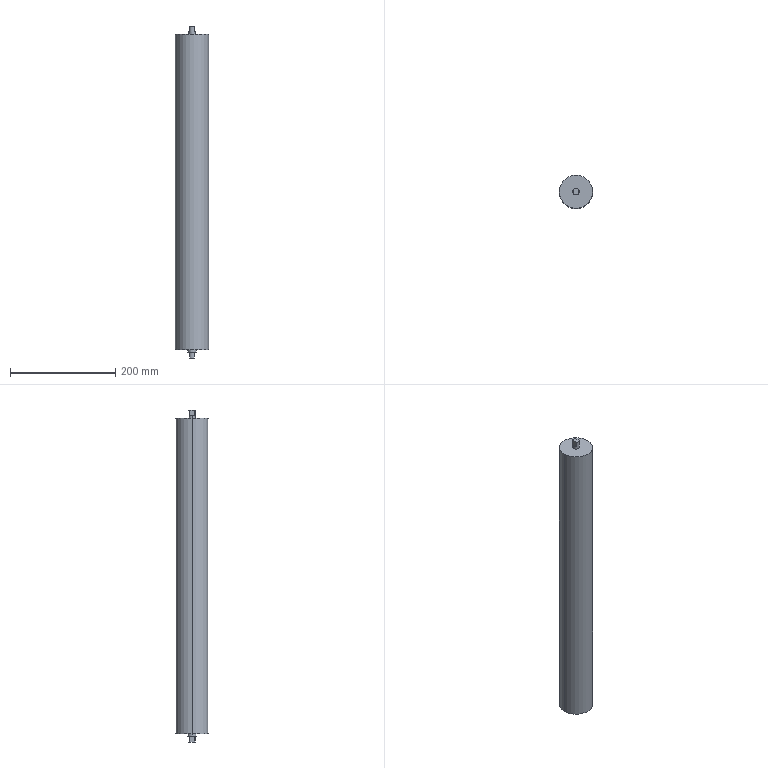Part | SolidWorks | features BaseBody 1 | 1 solid | 21 faces | box 63 x 63 x 632 mm | volume 1873911 mm3 | plane 13 | cylinder 8 | commonest cylinder face diameters 12 x4 16 x2 63 x2
STEP:
#1=CARTESIAN_POINT('',(-31.5,0.,300.));
#2=VERTEX_POINT('',#1);
#3=CARTESIAN_POINT('',(31.5,0.,300.));
#4=VERTEX_POINT('',#3);
#5=CARTESIAN_POINT('',(0.,0.,300.));
#6=DIRECTION('',(0.,0.,-1.));
#7=DIRECTION('',(-1.,0.,0.));
#8=AXIS2_PLACEMENT_3D('',#5,#6,#7);
#9=CIRCLE('',#8,31.5);
#10=EDGE_CURVE('',#2,#4,#9,.T.);
#11=ORIENTED_EDGE('',*,*,#10,.T.);
#12=CARTESIAN_POINT('',(31.5,0.,-300.));
#13=VERTEX_POINT('',#12);
#14=CARTESIAN_POINT('',(31.5,0.,300.));
#15=DIRECTION('',(0.,0.,-1.));
#16=VECTOR('',#15,1000.);
#17=LINE('',#14,#16);
#18=EDGE_CURVE('',#4,#13,#17,.T.);
#19=ORIENTED_EDGE('',*,*,#18,.T.);
#20=CARTESIAN_POINT('',(-31.5,0.,-300.));
#21=VERTEX_POINT('',#20);
#22=CARTESIAN_POINT('',(0.,0.,-300.));
#23=DIRECTION('',(0.,0.,1.));
#24=DIRECTION('',(-1.,0.,0.));
#25=AXIS2_PLACEMENT_3D('',#22,#23,#24);
#26=CIRCLE('',#25,31.5);
#27=EDGE_CURVE('',#13,#21,#26,.T.);
#28=ORIENTED_EDGE('',*,*,#27,.T.);
#29=CARTESIAN_POINT('',(-31.5,0.,300.));
#30=DIRECTION('',(0.,0.,-1.));
#31=VECTOR('',#30,1000.);
#32=LINE('',#29,#31);
#33=EDGE_CURVE('',#2,#21,#32,.T.);
#34=ORIENTED_EDGE('',*,*,#33,.F.);
#35=EDGE_LOOP('',(#11,#19,#28,#34));
#36=FACE_OUTER_BOUND('',#35,.T.);
#37=CARTESIAN_POINT('',(0.,0.,300.));
#38=DIRECTION('',(0.,0.,-1.));
#39=DIRECTION('',(-1.,0.,0.));
#40=AXIS2_PLACEMENT_3D('',#37,#38,#39);
#41=CYLINDRICAL_SURFACE('',#40,31.5);
#42=ADVANCED_FACE('',(#36),#41,.T.);
#43=CARTESIAN_POINT('',(8.,0.,-305.));
#44=VERTEX_POINT('',#43);
#45=CARTESIAN_POINT('',(-8.,0.,-305.));
#46=VERTEX_POINT('',#45);
#47=CARTESIAN_POINT('',(0.,0.,-305.));
#48=DIRECTION('',(0.,0.,1.));
#49=DIRECTION('',(1.,0.,0.));
#50=AXIS2_PLACEMENT_3D('',#47,#48,#49);
#51=CIRCLE('',#50,8.);
#52=EDGE_CURVE('',#44,#46,#51,.T.);
#53=ORIENTED_EDGE('',*,*,#52,.T.);
#54=CARTESIAN_POINT('',(-8.,0.,-300.));
#55=VERTEX_POINT('',#54);
#56=CARTESIAN_POINT('',(-8.,0.,-305.));
#57=DIRECTION('',(0.,0.,1.));
#58=VECTOR('',#57,1000.);
#59=LINE('',#56,#58);
#60=EDGE_CURVE('',#46,#55,#59,.T.);
#61=ORIENTED_EDGE('',*,*,#60,.T.);
#62=CARTESIAN_POINT('',(8.,0.,-300.));
#63=VERTEX_POINT('',#62);
#64=CARTESIAN_POINT('',(0.,0.,-300.));
#65=DIRECTION('',(0.,0.,-1.));
#66=DIRECTION('',(1.,0.,0.));
#67=AXIS2_PLACEMENT_3D('',#64,#65,#66);
#68=CIRCLE('',#67,8.);
#69=EDGE_CURVE('',#55,#63,#68,.T.);
#70=ORIENTED_EDGE('',*,*,#69,.T.);
#71=CARTESIAN_POINT('',(8.,0.,-305.));
#72=DIRECTION('',(0.,0.,1.));
#73=VECTOR('',#72,1000.);
#74=LINE('',#71,#73);
#75=EDGE_CURVE('',#44,#63,#74,.T.);
#76=ORIENTED_EDGE('',*,*,#75,.F.);
#77=EDGE_LOOP('',(#53,#61,#70,#76));
#78=FACE_OUTER_BOUND('',#77,.T.);
#79=CARTESIAN_POINT('',(0.,0.,-305.));
#80=DIRECTION('',(0.,0.,1.));
#81=DIRECTION('',(1.,0.,0.));
#82=AXIS2_PLACEMENT_3D('',#79,#80,#81);
#83=CYLINDRICAL_SURFACE('',#82,8.);
#84=ADVANCED_FACE('',(#78),#83,.T.);
#85=CARTESIAN_POINT('',(4.,4.472,306.));
#86=VERTEX_POINT('',#85);
#87=CARTESIAN_POINT('',(6.,0.,306.));
#88=VERTEX_POINT('',#87);
#89=CARTESIAN_POINT('',(0.,0.,306.));
#90=DIRECTION('',(0.,0.,-1.));
#91=DIRECTION('',(-1.,0.,0.));
#92=AXIS2_PLACEMENT_3D('',#89,#90,#91);
#93=CIRCLE('',#92,6.);
#94=EDGE_CURVE('',#86,#88,#93,.T.);
#95=ORIENTED_EDGE('',*,*,#94,.T.);
#96=CARTESIAN_POINT('',(6.,0.,300.));
#97=VERTEX_POINT('',#96);
#98=CARTESIAN_POINT('',(6.,0.,316.));
#99=DIRECTION('',(0.,0.,-1.));
#100=VECTOR('',#99,1000.);
#101=LINE('',#98,#100);
#102=EDGE_CURVE('',#88,#97,#101,.T.);
#103=ORIENTED_EDGE('',*,*,#102,.T.);
#104=CARTESIAN_POINT('',(-6.,0.,300.));
#105=VERTEX_POINT('',#104);
#106=CARTESIAN_POINT('',(0.,0.,300.));
#107=DIRECTION('',(0.,0.,-1.));
#108=DIRECTION('',(-1.,0.,0.));
#109=AXIS2_PLACEMENT_3D('',#106,#107,#108);
#110=CIRCLE('',#109,6.);
#111=EDGE_CURVE('',#105,#97,#110,.T.);
#112=ORIENTED_EDGE('',*,*,#111,.F.);
#113=CARTESIAN_POINT('',(-6.,0.,306.));
#114=VERTEX_POINT('',#113);
#115=CARTESIAN_POINT('',(-6.,0.,316.));
#116=DIRECTION('',(0.,0.,-1.));
#117=VECTOR('',#116,1000.);
#118=LINE('',#115,#117);
#119=EDGE_CURVE('',#114,#105,#118,.T.);
#120=ORIENTED_EDGE('',*,*,#119,.F.);
#121=CARTESIAN_POINT('',(-4.,4.472,306.));
#122=VERTEX_POINT('',#121);
#123=CARTESIAN_POINT('',(0.,0.,306.));
#124=DIRECTION('',(0.,0.,-1.));
#125=DIRECTION('',(-1.,0.,0.));
#126=AXIS2_PLACEMENT_3D('',#123,#124,#125);
#127=CIRCLE('',#126,6.);
#128=EDGE_CURVE('',#114,#122,#127,.T.);
#129=ORIENTED_EDGE('',*,*,#128,.T.);
#130=CARTESIAN_POINT('',(-4.,4.472,316.));
#131=VERTEX_POINT('',#130);
#132=CARTESIAN_POINT('',(-4.,4.472,316.));
#133=DIRECTION('',(0.,0.,1.));
#134=VECTOR('',#133,1000.);
#135=LINE('',#132,#134);
#136=EDGE_CURVE('',#122,#131,#135,.T.);
#137=ORIENTED_EDGE('',*,*,#136,.T.);
#138=CARTESIAN_POINT('',(4.,4.472,316.));
#139=VERTEX_POINT('',#138);
#140=CARTESIAN_POINT('',(0.,0.,316.));
#141=DIRECTION('',(0.,0.,-1.));
#142=DIRECTION('',(-1.,0.,0.));
#143=AXIS2_PLACEMENT_3D('',#140,#141,#142);
#144=CIRCLE('',#143,6.);
#145=EDGE_CURVE('',#131,#139,#144,.T.);
#146=ORIENTED_EDGE('',*,*,#145,.T.);
#147=CARTESIAN_POINT('',(4.,4.472,316.));
#148=DIRECTION('',(0.,0.,-1.));
#149=VECTOR('',#148,1000.);
#150=LINE('',#147,#149);
#151=EDGE_CURVE('',#139,#86,#150,.T.);
#152=ORIENTED_EDGE('',*,*,#151,.T.);
#153=EDGE_LOOP('',(#95,#103,#112,#120,#129,#137,#146,#152));
#154=FACE_OUTER_BOUND('',#153,.T.);
#155=CARTESIAN_POINT('',(0.,0.,316.));
#156=DIRECTION('',(0.,0.,-1.));
#157=DIRECTION('',(-1.,0.,0.));
#158=AXIS2_PLACEMENT_3D('',#155,#156,#157);
#159=CYLINDRICAL_SURFACE('',#158,6.);
#160=ADVANCED_FACE('',(#154),#159,.T.);
#161=CARTESIAN_POINT('',(-4.,4.472,-306.));
#162=VERTEX_POINT('',#161);
#163=CARTESIAN_POINT('',(-6.,0.,-306.));
#164=VERTEX_POINT('',#163);
#165=CARTESIAN_POINT('',(0.,0.,-306.));
#166=DIRECTION('',(0.,0.,1.));
#167=DIRECTION('',(1.,0.,0.));
#168=AXIS2_PLACEMENT_3D('',#165,#166,#167);
#169=CIRCLE('',#168,6.);
#170=EDGE_CURVE('',#162,#164,#169,.T.);
#171=ORIENTED_EDGE('',*,*,#170,.T.);
#172=CARTESIAN_POINT('',(-6.,0.,-305.));
#173=VERTEX_POINT('',#172);
#174=CARTESIAN_POINT('',(-6.,0.,-316.));
#175=DIRECTION('',(0.,0.,1.));
#176=VECTOR('',#175,1000.);
#177=LINE('',#174,#176);
#178=EDGE_CURVE('',#164,#173,#177,.T.);
#179=ORIENTED_EDGE('',*,*,#178,.T.);
#180=CARTESIAN_POINT('',(6.,0.,-305.));
#181=VERTEX_POINT('',#180);
#182=CARTESIAN_POINT('',(0.,0.,-305.));
#183=DIRECTION('',(0.,0.,1.));
#184=DIRECTION('',(1.,0.,0.));
#185=AXIS2_PLACEMENT_3D('',#182,#183,#184);
#186=CIRCLE('',#185,6.);
#187=EDGE_CURVE('',#181,#173,#186,.T.);
#188=ORIENTED_EDGE('',*,*,#187,.F.);
#189=CARTESIAN_POINT('',(6.,0.,-306.));
#190=VERTEX_POINT('',#189);
#191=CARTESIAN_POINT('',(6.,0.,-316.));
#192=DIRECTION('',(0.,0.,1.));
#193=VECTOR('',#192,1000.);
#194=LINE('',#191,#193);
#195=EDGE_CURVE('',#190,#181,#194,.T.);
#196=ORIENTED_EDGE('',*,*,#195,.F.);
#197=CARTESIAN_POINT('',(4.,4.472,-306.));
#198=VERTEX_POINT('',#197);
#199=CARTESIAN_POINT('',(0.,0.,-306.));
#200=DIRECTION('',(0.,0.,1.));
#201=DIRECTION('',(1.,0.,0.));
#202=AXIS2_PLACEMENT_3D('',#199,#200,#201);
#203=CIRCLE('',#202,6.);
#204=EDGE_CURVE('',#190,#198,#203,.T.);
#205=ORIENTED_EDGE('',*,*,#204,.T.);
#206=CARTESIAN_POINT('',(4.,4.472,-316.));
#207=VERTEX_POINT('',#206);
#208=CARTESIAN_POINT('',(4.,4.472,-316.));
#209=DIRECTION('',(0.,0.,-1.));
#210=VECTOR('',#209,1000.);
#211=LINE('',#208,#210);
#212=EDGE_CURVE('',#198,#207,#211,.T.);
#213=ORIENTED_EDGE('',*,*,#212,.T.);
#214=CARTESIAN_POINT('',(-4.,4.472,-316.));
#215=VERTEX_POINT('',#214);
#216=CARTESIAN_POINT('',(0.,0.,-316.));
#217=DIRECTION('',(0.,0.,1.));
#218=DIRECTION('',(1.,0.,0.));
#219=AXIS2_PLACEMENT_3D('',#216,#217,#218);
#220=CIRCLE('',#219,6.);
#221=EDGE_CURVE('',#207,#215,#220,.T.);
#222=ORIENTED_EDGE('',*,*,#221,.T.);
#223=CARTESIAN_POINT('',(-4.,4.472,-316.));
#224=DIRECTION('',(0.,0.,1.));
#225=VECTOR('',#224,1000.);
#226=LINE('',#223,#225);
#227=EDGE_CURVE('',#215,#162,#226,.T.);
#228=ORIENTED_EDGE('',*,*,#227,.T.);
#229=EDGE_LOOP('',(#171,#179,#188,#196,#205,#213,#222,#228));
#230=FACE_OUTER_BOUND('',#229,.T.);
#231=CARTESIAN_POINT('',(0.,0.,-316.));
#232=DIRECTION('',(0.,0.,1.));
#233=DIRECTION('',(1.,0.,0.));
#234=AXIS2_PLACEMENT_3D('',#231,#232,#233);
#235=CYLINDRICAL_SURFACE('',#234,6.);
#236=ADVANCED_FACE('',(#230),#235,.T.);
#237=ORIENTED_EDGE('',*,*,#18,.F.);
#238=CARTESIAN_POINT('',(0.,0.,300.));
#239=DIRECTION('',(0.,0.,-1.));
#240=DIRECTION('',(-1.,0.,0.));
#241=AXIS2_PLACEMENT_3D('',#238,#239,#240);
#242=CIRCLE('',#241,31.5);
#243=EDGE_CURVE('',#4,#2,#242,.T.);
#244=ORIENTED_EDGE('',*,*,#243,.T.);
#245=ORIENTED_EDGE('',*,*,#33,.T.);
#246=CARTESIAN_POINT('',(0.,0.,-300.));
#247=DIRECTION('',(0.,0.,1.));
#248=DIRECTION('',(-1.,0.,0.));
#249=AXIS2_PLACEMENT_3D('',#246,#247,#248);
#250=CIRCLE('',#249,31.5);
#251=EDGE_CURVE('',#21,#13,#250,.T.);
#252=ORIENTED_EDGE('',*,*,#251,.T.);
#253=EDGE_LOOP('',(#237,#244,#245,#252));
#254=FACE_OUTER_BOUND('',#253,.T.);
#255=CARTESIAN_POINT('',(0.,0.,300.));
#256=DIRECTION('',(0.,0.,-1.));
#257=DIRECTION('',(-1.,0.,0.));
#258=AXIS2_PLACEMENT_3D('',#255,#256,#257);
#259=CYLINDRICAL_SURFACE('',#258,31.5);
#260=ADVANCED_FACE('',(#254),#259,.T.);
#261=CARTESIAN_POINT('',(0.,0.,-300.));
#262=DIRECTION('',(0.,0.,-1.));
#263=DIRECTION('',(1.,0.,0.));
#264=AXIS2_PLACEMENT_3D('',#261,#262,#263);
#265=CIRCLE('',#264,8.);
#266=EDGE_CURVE('',#63,#55,#265,.T.);
#267=ORIENTED_EDGE('',*,*,#266,.F.);
#268=ORIENTED_EDGE('',*,*,#69,.F.);
#269=EDGE_LOOP('',(#267,#268));
#270=FACE_BOUND('',#269,.T.);
#271=ORIENTED_EDGE('',*,*,#251,.F.);
#272=ORIENTED_EDGE('',*,*,#27,.F.);
#273=EDGE_LOOP('',(#271,#272));
#274=FACE_OUTER_BOUND('',#273,.T.);
#275=CARTESIAN_POINT('',(0.,0.,-300.));
#276=DIRECTION('',(0.,0.,1.));
#277=DIRECTION('',(1.,0.,0.));
#278=AXIS2_PLACEMENT_3D('',#275,#276,#277);
#279=PLANE('',#278);
#280=ADVANCED_FACE('',(#270,#274),#279,.F.);
#281=ORIENTED_EDGE('',*,*,#10,.F.);
#282=ORIENTED_EDGE('',*,*,#243,.F.);
#283=EDGE_LOOP('',(#281,#282));
#284=FACE_OUTER_BOUND('',#283,.T.);
#285=ORIENTED_EDGE('',*,*,#111,.T.);
#286=CARTESIAN_POINT('',(0.,0.,300.));
#287=DIRECTION('',(0.,0.,-1.));
#288=DIRECTION('',(-1.,0.,0.));
#289=AXIS2_PLACEMENT_3D('',#286,#287,#288);
#290=CIRCLE('',#289,6.);
#291=EDGE_CURVE('',#97,#105,#290,.T.);
#292=ORIENTED_EDGE('',*,*,#291,.T.);
#293=EDGE_LOOP('',(#285,#292));
#294=FACE_BOUND('',#293,.T.);
#295=CARTESIAN_POINT('',(0.,0.,300.));
#296=DIRECTION('',(0.,0.,1.));
#297=DIRECTION('',(1.,0.,0.));
#298=AXIS2_PLACEMENT_3D('',#295,#296,#297);
#299=PLANE('',#298);
#300=ADVANCED_FACE('',(#284,#294),#299,.T.);
#301=ORIENTED_EDGE('',*,*,#60,.F.);
#302=CARTESIAN_POINT('',(0.,0.,-305.));
#303=DIRECTION('',(0.,0.,1.));
#304=DIRECTION('',(1.,0.,0.));
#305=AXIS2_PLACEMENT_3D('',#302,#303,#304);
#306=CIRCLE('',#305,8.);
#307=EDGE_CURVE('',#46,#44,#306,.T.);
#308=ORIENTED_EDGE('',*,*,#307,.T.);
#309=ORIENTED_EDGE('',*,*,#75,.T.);
#310=ORIENTED_EDGE('',*,*,#266,.T.);
#311=EDGE_LOOP('',(#301,#308,#309,#310));
#312=FACE_OUTER_BOUND('',#311,.T.);
#313=CARTESIAN_POINT('',(0.,0.,-305.));
#314=DIRECTION('',(0.,0.,1.));
#315=DIRECTION('',(1.,0.,0.));
#316=AXIS2_PLACEMENT_3D('',#313,#314,#315);
#317=CYLINDRICAL_SURFACE('',#316,8.);
#318=ADVANCED_FACE('',(#312),#317,.T.);
#319=ORIENTED_EDGE('',*,*,#102,.F.);
#320=CARTESIAN_POINT('',(4.,-4.472,306.));
#321=VERTEX_POINT('',#320);
#322=CARTESIAN_POINT('',(0.,0.,306.));
#323=DIRECTION('',(0.,0.,-1.));
#324=DIRECTION('',(-1.,0.,0.));
#325=AXIS2_PLACEMENT_3D('',#322,#323,#324);
#326=CIRCLE('',#325,6.);
#327=EDGE_CURVE('',#88,#321,#326,.T.);
#328=ORIENTED_EDGE('',*,*,#327,.T.);
#329=CARTESIAN_POINT('',(4.,-4.472,316.));
#330=VERTEX_POINT('',#329);
#331=CARTESIAN_POINT('',(4.,-4.472,316.));
#332=DIRECTION('',(0.,0.,1.));
#333=VECTOR('',#332,1000.);
#334=LINE('',#331,#333);
#335=EDGE_CURVE('',#321,#330,#334,.T.);
#336=ORIENTED_EDGE('',*,*,#335,.T.);
#337=CARTESIAN_POINT('',(-4.,-4.472,316.));
#338=VERTEX_POINT('',#337);
#339=CARTESIAN_POINT('',(0.,0.,316.));
#340=DIRECTION('',(0.,0.,-1.));
#341=DIRECTION('',(-1.,0.,0.));
#342=AXIS2_PLACEMENT_3D('',#339,#340,#341);
#343=CIRCLE('',#342,6.);
#344=EDGE_CURVE('',#330,#338,#343,.T.);
#345=ORIENTED_EDGE('',*,*,#344,.T.);
#346=CARTESIAN_POINT('',(-4.,-4.472,306.));
#347=VERTEX_POINT('',#346);
#348=CARTESIAN_POINT('',(-4.,-4.472,316.));
#349=DIRECTION('',(0.,0.,-1.));
#350=VECTOR('',#349,1000.);
#351=LINE('',#348,#350);
#352=EDGE_CURVE('',#338,#347,#351,.T.);
#353=ORIENTED_EDGE('',*,*,#352,.T.);
#354=CARTESIAN_POINT('',(0.,0.,306.));
#355=DIRECTION('',(0.,0.,-1.));
#356=DIRECTION('',(-1.,0.,0.));
#357=AXIS2_PLACEMENT_3D('',#354,#355,#356);
#358=CIRCLE('',#357,6.);
#359=EDGE_CURVE('',#347,#114,#358,.T.);
#360=ORIENTED_EDGE('',*,*,#359,.T.);
#361=ORIENTED_EDGE('',*,*,#119,.T.);
#362=ORIENTED_EDGE('',*,*,#291,.F.);
#363=EDGE_LOOP('',(#319,#328,#336,#345,#353,#360,#361,#362));
#364=FACE_OUTER_BOUND('',#363,.T.);
#365=CARTESIAN_POINT('',(0.,0.,316.));
#366=DIRECTION('',(0.,0.,-1.));
#367=DIRECTION('',(-1.,0.,0.));
#368=AXIS2_PLACEMENT_3D('',#365,#366,#367);
#369=CYLINDRICAL_SURFACE('',#368,6.);
#370=ADVANCED_FACE('',(#364),#369,.T.);
#371=ORIENTED_EDGE('',*,*,#187,.T.);
#372=CARTESIAN_POINT('',(0.,0.,-305.));
#373=DIRECTION('',(0.,0.,1.));
#374=DIRECTION('',(1.,0.,0.));
#375=AXIS2_PLACEMENT_3D('',#372,#373,#374);
#376=CIRCLE('',#375,6.);
#377=EDGE_CURVE('',#173,#181,#376,.T.);
#378=ORIENTED_EDGE('',*,*,#377,.T.);
#379=EDGE_LOOP('',(#371,#378));
#380=FACE_BOUND('',#379,.T.);
#381=ORIENTED_EDGE('',*,*,#52,.F.);
#382=ORIENTED_EDGE('',*,*,#307,.F.);
#383=EDGE_LOOP('',(#381,#382));
#384=FACE_OUTER_BOUND('',#383,.T.);
#385=CARTESIAN_POINT('',(0.,0.,-305.));
#386=DIRECTION('',(0.,0.,-1.));
#387=DIRECTION('',(-1.,0.,0.));
#388=AXIS2_PLACEMENT_3D('',#385,#386,#387);
#389=PLANE('',#388);
#390=ADVANCED_FACE('',(#380,#384),#389,.T.);
#391=CARTESIAN_POINT('',(4.,8.62,316.));
#392=DIRECTION('',(0.,1.,0.));
#393=VECTOR('',#392,1000.);
#394=LINE('',#391,#393);
#395=EDGE_CURVE('',#330,#139,#394,.T.);
#396=ORIENTED_EDGE('',*,*,#395,.F.);
#397=ORIENTED_EDGE('',*,*,#335,.F.);
#398=CARTESIAN_POINT('',(4.,8.62,306.));
#399=DIRECTION('',(0.,-1.,0.));
#400=VECTOR('',#399,1000.);
#401=LINE('',#398,#400);
#402=EDGE_CURVE('',#86,#321,#401,.T.);
#403=ORIENTED_EDGE('',*,*,#402,.F.);
#404=ORIENTED_EDGE('',*,*,#151,.F.);
#405=EDGE_LOOP('',(#396,#397,#403,#404));
#406=FACE_OUTER_BOUND('',#405,.T.);
#407=CARTESIAN_POINT('',(4.,8.62,306.));
#408=DIRECTION('',(-1.,0.,0.));
#409=DIRECTION('',(0.,-1.,0.));
#410=AXIS2_PLACEMENT_3D('',#407,#408,#409);
#411=PLANE('',#410);
#412=ADVANCED_FACE('',(#406),#411,.F.);
#413=ORIENTED_EDGE('',*,*,#395,.T.);
#414=ORIENTED_EDGE('',*,*,#145,.F.);
#415=CARTESIAN_POINT('',(-4.,0.,316.));
#416=DIRECTION('',(0.,-1.,0.));
#417=VECTOR('',#416,1000.);
#418=LINE('',#415,#417);
#419=EDGE_CURVE('',#131,#338,#418,.T.);
#420=ORIENTED_EDGE('',*,*,#419,.T.);
#421=ORIENTED_EDGE('',*,*,#344,.F.);
#422=EDGE_LOOP('',(#413,#414,#420,#421));
#423=FACE_OUTER_BOUND('',#422,.T.);
#424=CARTESIAN_POINT('',(0.,0.,316.));
#425=DIRECTION('',(0.,0.,1.));
#426=DIRECTION('',(1.,0.,0.));
#427=AXIS2_PLACEMENT_3D('',#424,#425,#426);
#428=PLANE('',#427);
#429=ADVANCED_FACE('',(#423),#428,.T.);
#430=ORIENTED_EDGE('',*,*,#419,.F.);
#431=ORIENTED_EDGE('',*,*,#136,.F.);
#432=CARTESIAN_POINT('',(-4.,8.62,306.));
#433=DIRECTION('',(0.,1.,0.));
#434=VECTOR('',#433,1000.);
#435=LINE('',#432,#434);
#436=EDGE_CURVE('',#347,#122,#435,.T.);
#437=ORIENTED_EDGE('',*,*,#436,.F.);
#438=ORIENTED_EDGE('',*,*,#352,.F.);
#439=EDGE_LOOP('',(#430,#431,#437,#438));
#440=FACE_OUTER_BOUND('',#439,.T.);
#441=CARTESIAN_POINT('',(-4.,8.62,306.));
#442=DIRECTION('',(1.,0.,0.));
#443=DIRECTION('',(0.,1.,0.));
#444=AXIS2_PLACEMENT_3D('',#441,#442,#443);
#445=PLANE('',#444);
#446=ADVANCED_FACE('',(#440),#445,.F.);
#447=ORIENTED_EDGE('',*,*,#359,.F.);
#448=ORIENTED_EDGE('',*,*,#436,.T.);
#449=ORIENTED_EDGE('',*,*,#128,.F.);
#450=EDGE_LOOP('',(#447,#448,#449));
#451=FACE_OUTER_BOUND('',#450,.T.);
#452=CARTESIAN_POINT('',(0.,0.,306.));
#453=DIRECTION('',(0.,0.,1.));
#454=DIRECTION('',(1.,0.,0.));
#455=AXIS2_PLACEMENT_3D('',#452,#453,#454);
#456=PLANE('',#455);
#457=ADVANCED_FACE('',(#451),#456,.T.);
#458=ORIENTED_EDGE('',*,*,#402,.T.);
#459=ORIENTED_EDGE('',*,*,#327,.F.);
#460=ORIENTED_EDGE('',*,*,#94,.F.);
#461=EDGE_LOOP('',(#458,#459,#460));
#462=FACE_OUTER_BOUND('',#461,.T.);
#463=CARTESIAN_POINT('',(0.,0.,306.));
#464=DIRECTION('',(0.,0.,1.));
#465=DIRECTION('',(1.,0.,0.));
#466=AXIS2_PLACEMENT_3D('',#463,#464,#465);
#467=PLANE('',#466);
#468=ADVANCED_FACE('',(#462),#467,.T.);
#469=ORIENTED_EDGE('',*,*,#178,.F.);
#470=CARTESIAN_POINT('',(-4.,-4.472,-306.));
#471=VERTEX_POINT('',#470);
#472=CARTESIAN_POINT('',(0.,0.,-306.));
#473=DIRECTION('',(0.,0.,1.));
#474=DIRECTION('',(1.,0.,0.));
#475=AXIS2_PLACEMENT_3D('',#472,#473,#474);
#476=CIRCLE('',#475,6.);
#477=EDGE_CURVE('',#164,#471,#476,.T.);
#478=ORIENTED_EDGE('',*,*,#477,.T.);
#479=CARTESIAN_POINT('',(-4.,-4.472,-316.));
#480=VERTEX_POINT('',#479);
#481=CARTESIAN_POINT('',(-4.,-4.472,-316.));
#482=DIRECTION('',(0.,0.,-1.));
#483=VECTOR('',#482,1000.);
#484=LINE('',#481,#483);
#485=EDGE_CURVE('',#471,#480,#484,.T.);
#486=ORIENTED_EDGE('',*,*,#485,.T.);
#487=CARTESIAN_POINT('',(4.,-4.472,-316.));
#488=VERTEX_POINT('',#487);
#489=CARTESIAN_POINT('',(0.,0.,-316.));
#490=DIRECTION('',(0.,0.,1.));
#491=DIRECTION('',(1.,0.,0.));
#492=AXIS2_PLACEMENT_3D('',#489,#490,#491);
#493=CIRCLE('',#492,6.);
#494=EDGE_CURVE('',#480,#488,#493,.T.);
#495=ORIENTED_EDGE('',*,*,#494,.T.);
#496=CARTESIAN_POINT('',(4.,-4.472,-306.));
#497=VERTEX_POINT('',#496);
#498=CARTESIAN_POINT('',(4.,-4.472,-316.));
#499=DIRECTION('',(0.,0.,1.));
#500=VECTOR('',#499,1000.);
#501=LINE('',#498,#500);
#502=EDGE_CURVE('',#488,#497,#501,.T.);
#503=ORIENTED_EDGE('',*,*,#502,.T.);
#504=CARTESIAN_POINT('',(0.,0.,-306.));
#505=DIRECTION('',(0.,0.,1.));
#506=DIRECTION('',(1.,0.,0.));
#507=AXIS2_PLACEMENT_3D('',#504,#505,#506);
#508=CIRCLE('',#507,6.);
#509=EDGE_CURVE('',#497,#190,#508,.T.);
#510=ORIENTED_EDGE('',*,*,#509,.T.);
#511=ORIENTED_EDGE('',*,*,#195,.T.);
#512=ORIENTED_EDGE('',*,*,#377,.F.);
#513=EDGE_LOOP('',(#469,#478,#486,#495,#503,#510,#511,#512));
#514=FACE_OUTER_BOUND('',#513,.T.);
#515=CARTESIAN_POINT('',(0.,0.,-316.));
#516=DIRECTION('',(0.,0.,1.));
#517=DIRECTION('',(1.,0.,0.));
#518=AXIS2_PLACEMENT_3D('',#515,#516,#517);
#519=CYLINDRICAL_SURFACE('',#518,6.);
#520=ADVANCED_FACE('',(#514),#519,.T.);
#521=ORIENTED_EDGE('',*,*,#509,.F.);
#522=CARTESIAN_POINT('',(4.,0.,-306.));
#523=DIRECTION('',(0.,1.,0.));
#524=VECTOR('',#523,1000.);
#525=LINE('',#522,#524);
#526=EDGE_CURVE('',#497,#198,#525,.T.);
#527=ORIENTED_EDGE('',*,*,#526,.T.);
#528=ORIENTED_EDGE('',*,*,#204,.F.);
#529=EDGE_LOOP('',(#521,#527,#528));
#530=FACE_OUTER_BOUND('',#529,.T.);
#531=CARTESIAN_POINT('',(0.,0.,-306.));
#532=DIRECTION('',(0.,0.,-1.));
#533=DIRECTION('',(-1.,0.,0.));
#534=AXIS2_PLACEMENT_3D('',#531,#532,#533);
#535=PLANE('',#534);
#536=ADVANCED_FACE('',(#530),#535,.T.);
#537=ORIENTED_EDGE('',*,*,#502,.F.);
#538=CARTESIAN_POINT('',(4.,8.62,-316.));
#539=DIRECTION('',(0.,1.,0.));
#540=VECTOR('',#539,1000.);
#541=LINE('',#538,#540);
#542=EDGE_CURVE('',#488,#207,#541,.T.);
#543=ORIENTED_EDGE('',*,*,#542,.T.);
#544=ORIENTED_EDGE('',*,*,#212,.F.);
#545=ORIENTED_EDGE('',*,*,#526,.F.);
#546=EDGE_LOOP('',(#537,#543,#544,#545));
#547=FACE_OUTER_BOUND('',#546,.T.);
#548=CARTESIAN_POINT('',(4.,8.62,-306.));
#549=DIRECTION('',(1.,0.,0.));
#550=DIRECTION('',(0.,1.,0.));
#551=AXIS2_PLACEMENT_3D('',#548,#549,#550);
#552=PLANE('',#551);
#553=ADVANCED_FACE('',(#547),#552,.T.);
#554=ORIENTED_EDGE('',*,*,#221,.F.);
#555=ORIENTED_EDGE('',*,*,#542,.F.);
#556=ORIENTED_EDGE('',*,*,#494,.F.);
#557=CARTESIAN_POINT('',(-4.,0.,-316.));
#558=DIRECTION('',(0.,1.,0.));
#559=VECTOR('',#558,1000.);
#560=LINE('',#557,#559);
#561=EDGE_CURVE('',#480,#215,#560,.T.);
#562=ORIENTED_EDGE('',*,*,#561,.T.);
#563=EDGE_LOOP('',(#554,#555,#556,#562));
#564=FACE_OUTER_BOUND('',#563,.T.);
#565=CARTESIAN_POINT('',(0.,0.,-316.));
#566=DIRECTION('',(0.,0.,-1.));
#567=DIRECTION('',(-1.,0.,0.));
#568=AXIS2_PLACEMENT_3D('',#565,#566,#567);
#569=PLANE('',#568);
#570=ADVANCED_FACE('',(#564),#569,.T.);
#571=ORIENTED_EDGE('',*,*,#227,.F.);
#572=ORIENTED_EDGE('',*,*,#561,.F.);
#573=ORIENTED_EDGE('',*,*,#485,.F.);
#574=CARTESIAN_POINT('',(-4.,8.62,-306.));
#575=DIRECTION('',(0.,1.,0.));
#576=VECTOR('',#575,1000.);
#577=LINE('',#574,#576);
#578=EDGE_CURVE('',#471,#162,#577,.T.);
#579=ORIENTED_EDGE('',*,*,#578,.T.);
#580=EDGE_LOOP('',(#571,#572,#573,#579));
#581=FACE_OUTER_BOUND('',#580,.T.);
#582=CARTESIAN_POINT('',(-4.,8.62,-306.));
#583=DIRECTION('',(-1.,0.,0.));
#584=DIRECTION('',(0.,-1.,0.));
#585=AXIS2_PLACEMENT_3D('',#582,#583,#584);
#586=PLANE('',#585);
#587=ADVANCED_FACE('',(#581),#586,.T.);
#588=ORIENTED_EDGE('',*,*,#170,.F.);
#589=ORIENTED_EDGE('',*,*,#578,.F.);
#590=ORIENTED_EDGE('',*,*,#477,.F.);
#591=EDGE_LOOP('',(#588,#589,#590));
#592=FACE_OUTER_BOUND('',#591,.T.);
#593=CARTESIAN_POINT('',(0.,0.,-306.));
#594=DIRECTION('',(0.,0.,-1.));
#595=DIRECTION('',(-1.,0.,0.));
#596=AXIS2_PLACEMENT_3D('',#593,#594,#595);
#597=PLANE('',#596);
#598=ADVANCED_FACE('',(#592),#597,.T.);
#599=CLOSED_SHELL('',(#42,#84,#160,#236,#260,#280,#300,#318,#370,#390,#412,#429,#446,#457,#468,#520,#536,#553,#570,#587,#598));
#600=MANIFOLD_SOLID_BREP('',#599);
#601=CARTESIAN_POINT('',(0.,0.,0.));
#602=DIRECTION('',(0.,0.,1.));
#603=DIRECTION('',(1.,0.,0.));
#604=AXIS2_PLACEMENT_3D('',#601,#602,#603);
#605=(LENGTH_UNIT()NAMED_UNIT(*)SI_UNIT(.MILLI.,.METRE.));
#606=UNCERTAINTY_MEASURE_WITH_UNIT(LENGTH_MEASURE(0.00001),#605,'','');
#607=(NAMED_UNIT(*)PLANE_ANGLE_UNIT()SI_UNIT($,.RADIAN.));
#608=(NAMED_UNIT(*)SI_UNIT($,.STERADIAN.)SOLID_ANGLE_UNIT());
#609=(GEOMETRIC_REPRESENTATION_CONTEXT(3)GLOBAL_UNCERTAINTY_ASSIGNED_CONTEXT((#606))GLOBAL_UNIT_ASSIGNED_CONTEXT((#605,#607,#608))REPRESENTATION_CONTEXT('',''));
#610=ADVANCED_BREP_SHAPE_REPRESENTATION('',(#600,#604),#609);